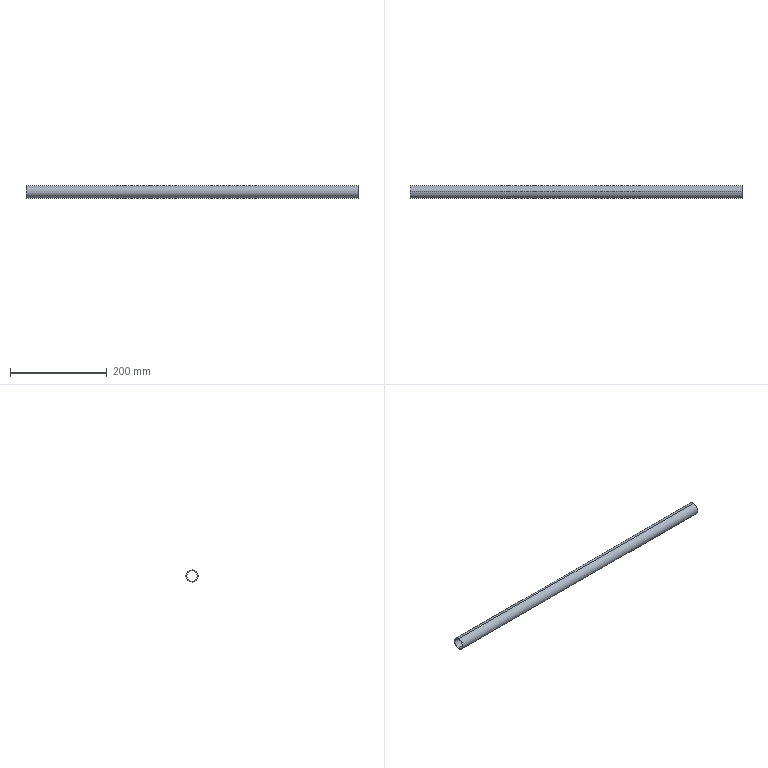Part | STEP file | E3-中转釜护栏7栏杆_Default<As Machined> | 1 solid | 6 faces | box 685 x 25 x 25 mm | volume 75858 mm3 | cylinder 4 | plane 2 | commonest cylinder face diameters 22 x2 25 x2
STEP:
#1=CARTESIAN_POINT('',(0.,0.,0.));
#2=DIRECTION('',(0.,0.,1.));
#3=DIRECTION('',(1.,0.,0.));
#4=AXIS2_PLACEMENT_3D('',#1,#2,#3);
#5=CARTESIAN_POINT('',(0.,0.,-12.5));
#6=VERTEX_POINT('',#5);
#7=CARTESIAN_POINT('',(0.,0.,12.5));
#8=VERTEX_POINT('',#7);
#9=CARTESIAN_POINT('',(0.,0.,0.));
#10=DIRECTION('',(-1.,0.,0.));
#11=DIRECTION('',(0.,0.,1.));
#12=AXIS2_PLACEMENT_3D('',#9,#10,#11);
#13=CIRCLE('',#12,12.5);
#14=CARTESIAN_POINT('',(0.,0.,0.));
#15=DIRECTION('',(-1.,0.,0.));
#16=DIRECTION('',(0.,0.,-1.));
#17=AXIS2_PLACEMENT_3D('',#14,#15,#16);
#18=CYLINDRICAL_SURFACE('',#17,12.5);
#19=CARTESIAN_POINT('',(-3.142,0.));
#20=DIRECTION('',(1.,0.));
#21=VECTOR('',#20,1.);
#22=LINE('',#19,#21);
#23=(GEOMETRIC_REPRESENTATION_CONTEXT(2)PARAMETRIC_REPRESENTATION_CONTEXT()REPRESENTATION_CONTEXT('',''));
#24=DEFINITIONAL_REPRESENTATION('',(#22),#23);
#25=PCURVE('',#18,#24);
#26=CARTESIAN_POINT('',(0.,0.,0.));
#27=DIRECTION('',(1.,0.,0.));
#28=DIRECTION('',(0.,0.,1.));
#29=AXIS2_PLACEMENT_3D('',#26,#27,#28);
#30=PLANE('',#29);
#31=CARTESIAN_POINT('',(12.5,0.));
#32=CARTESIAN_POINT('',(12.5,-21.651));
#33=CARTESIAN_POINT('',(-6.25,-10.825));
#34=CARTESIAN_POINT('',(-25.,0.));
#35=CARTESIAN_POINT('',(-6.25,10.825));
#36=CARTESIAN_POINT('',(12.5,21.651));
#37=CARTESIAN_POINT('',(12.5,0.));
#38=(BOUNDED_CURVE()B_SPLINE_CURVE(2,(#31,#32,#33,#34,#35,#36,#37),.UNSPECIFIED.,.T.,.F.)B_SPLINE_CURVE_WITH_KNOTS((1,2,2,2,2,1),(-2.094,0.,2.094,4.189,6.283,8.378),.UNSPECIFIED.)CURVE()GEOMETRIC_REPRESENTATION_ITEM()RATIONAL_B_SPLINE_CURVE((1.,0.5,1.,0.5,1.,0.5,1.))REPRESENTATION_ITEM(''));
#39=(GEOMETRIC_REPRESENTATION_CONTEXT(2)PARAMETRIC_REPRESENTATION_CONTEXT()REPRESENTATION_CONTEXT('',''));
#40=DEFINITIONAL_REPRESENTATION('',(#38),#39);
#41=PCURVE('',#30,#40);
#42=SURFACE_CURVE('',#13,(#25,#41),.PCURVE_S1.);
#43=EDGE_CURVE('',#6,#8,#42,.T.);
#44=ORIENTED_EDGE('',*,*,#43,.T.);
#45=CARTESIAN_POINT('',(-685.,0.,12.5));
#46=VERTEX_POINT('',#45);
#47=CARTESIAN_POINT('',(0.,0.,12.5));
#48=DIRECTION('',(-1.,0.,0.));
#49=VECTOR('',#48,1.);
#50=LINE('',#47,#49);
#51=CARTESIAN_POINT('',(3.142,0.));
#52=DIRECTION('',(0.,1.));
#53=VECTOR('',#52,1.);
#54=LINE('',#51,#53);
#55=(GEOMETRIC_REPRESENTATION_CONTEXT(2)PARAMETRIC_REPRESENTATION_CONTEXT()REPRESENTATION_CONTEXT('',''));
#56=DEFINITIONAL_REPRESENTATION('',(#54),#55);
#57=PCURVE('',#18,#56);
#58=CARTESIAN_POINT('',(0.,0.,0.));
#59=DIRECTION('',(-1.,0.,0.));
#60=DIRECTION('',(0.,0.,-1.));
#61=AXIS2_PLACEMENT_3D('',#58,#59,#60);
#62=CYLINDRICAL_SURFACE('',#61,12.5);
#63=CARTESIAN_POINT('',(3.142,0.));
#64=DIRECTION('',(0.,1.));
#65=VECTOR('',#64,1.);
#66=LINE('',#63,#65);
#67=(GEOMETRIC_REPRESENTATION_CONTEXT(2)PARAMETRIC_REPRESENTATION_CONTEXT()REPRESENTATION_CONTEXT('',''));
#68=DEFINITIONAL_REPRESENTATION('',(#66),#67);
#69=PCURVE('',#62,#68);
#70=SURFACE_CURVE('',#50,(#57,#69),.PCURVE_S1.);
#71=EDGE_CURVE('',#8,#46,#70,.T.);
#72=ORIENTED_EDGE('',*,*,#71,.T.);
#73=CARTESIAN_POINT('',(-685.,0.,-12.5));
#74=VERTEX_POINT('',#73);
#75=CARTESIAN_POINT('',(-685.,0.,0.));
#76=DIRECTION('',(-1.,0.,0.));
#77=DIRECTION('',(0.,0.,1.));
#78=AXIS2_PLACEMENT_3D('',#75,#76,#77);
#79=CIRCLE('',#78,12.5);
#80=CARTESIAN_POINT('',(-3.142,685.));
#81=DIRECTION('',(1.,0.));
#82=VECTOR('',#81,1.);
#83=LINE('',#80,#82);
#84=(GEOMETRIC_REPRESENTATION_CONTEXT(2)PARAMETRIC_REPRESENTATION_CONTEXT()REPRESENTATION_CONTEXT('',''));
#85=DEFINITIONAL_REPRESENTATION('',(#83),#84);
#86=PCURVE('',#18,#85);
#87=CARTESIAN_POINT('',(-685.,0.,0.));
#88=DIRECTION('',(1.,0.,0.));
#89=DIRECTION('',(0.,0.,1.));
#90=AXIS2_PLACEMENT_3D('',#87,#88,#89);
#91=PLANE('',#90);
#92=CARTESIAN_POINT('',(12.5,0.));
#93=CARTESIAN_POINT('',(12.5,-21.651));
#94=CARTESIAN_POINT('',(-6.25,-10.825));
#95=CARTESIAN_POINT('',(-25.,0.));
#96=CARTESIAN_POINT('',(-6.25,10.825));
#97=CARTESIAN_POINT('',(12.5,21.651));
#98=CARTESIAN_POINT('',(12.5,0.));
#99=(BOUNDED_CURVE()B_SPLINE_CURVE(2,(#92,#93,#94,#95,#96,#97,#98),.UNSPECIFIED.,.T.,.F.)B_SPLINE_CURVE_WITH_KNOTS((1,2,2,2,2,1),(-2.094,0.,2.094,4.189,6.283,8.378),.UNSPECIFIED.)CURVE()GEOMETRIC_REPRESENTATION_ITEM()RATIONAL_B_SPLINE_CURVE((1.,0.5,1.,0.5,1.,0.5,1.))REPRESENTATION_ITEM(''));
#100=(GEOMETRIC_REPRESENTATION_CONTEXT(2)PARAMETRIC_REPRESENTATION_CONTEXT()REPRESENTATION_CONTEXT('',''));
#101=DEFINITIONAL_REPRESENTATION('',(#99),#100);
#102=PCURVE('',#91,#101);
#103=SURFACE_CURVE('',#79,(#86,#102),.PCURVE_S1.);
#104=EDGE_CURVE('',#74,#46,#103,.T.);
#105=ORIENTED_EDGE('',*,*,#104,.F.);
#106=CARTESIAN_POINT('',(0.,0.,-12.5));
#107=DIRECTION('',(-1.,0.,0.));
#108=VECTOR('',#107,1.);
#109=LINE('',#106,#108);
#110=CARTESIAN_POINT('',(0.,0.));
#111=DIRECTION('',(0.,1.));
#112=VECTOR('',#111,1.);
#113=LINE('',#110,#112);
#114=(GEOMETRIC_REPRESENTATION_CONTEXT(2)PARAMETRIC_REPRESENTATION_CONTEXT()REPRESENTATION_CONTEXT('',''));
#115=DEFINITIONAL_REPRESENTATION('',(#113),#114);
#116=PCURVE('',#18,#115);
#117=CARTESIAN_POINT('',(6.283,0.));
#118=DIRECTION('',(0.,1.));
#119=VECTOR('',#118,1.);
#120=LINE('',#117,#119);
#121=(GEOMETRIC_REPRESENTATION_CONTEXT(2)PARAMETRIC_REPRESENTATION_CONTEXT()REPRESENTATION_CONTEXT('',''));
#122=DEFINITIONAL_REPRESENTATION('',(#120),#121);
#123=PCURVE('',#62,#122);
#124=SURFACE_CURVE('',#109,(#116,#123),.PCURVE_S1.);
#125=EDGE_CURVE('',#6,#74,#124,.T.);
#126=ORIENTED_EDGE('',*,*,#125,.F.);
#127=EDGE_LOOP('',(#44,#72,#105,#126));
#128=FACE_BOUND('',#127,.T.);
#129=ADVANCED_FACE('',(#128),#18,.T.);
#130=CARTESIAN_POINT('',(0.,0.,-11.));
#131=VERTEX_POINT('',#130);
#132=CARTESIAN_POINT('',(-685.,0.,-11.));
#133=VERTEX_POINT('',#132);
#134=CARTESIAN_POINT('',(0.,0.,-11.));
#135=DIRECTION('',(-1.,0.,0.));
#136=VECTOR('',#135,1.);
#137=LINE('',#134,#136);
#138=CARTESIAN_POINT('',(0.,0.,0.));
#139=DIRECTION('',(-1.,0.,0.));
#140=DIRECTION('',(0.,0.,-1.));
#141=AXIS2_PLACEMENT_3D('',#138,#139,#140);
#142=CYLINDRICAL_SURFACE('',#141,11.);
#143=CARTESIAN_POINT('',(6.283,0.));
#144=DIRECTION('',(0.,1.));
#145=VECTOR('',#144,1.);
#146=LINE('',#143,#145);
#147=(GEOMETRIC_REPRESENTATION_CONTEXT(2)PARAMETRIC_REPRESENTATION_CONTEXT()REPRESENTATION_CONTEXT('',''));
#148=DEFINITIONAL_REPRESENTATION('',(#146),#147);
#149=PCURVE('',#142,#148);
#150=CARTESIAN_POINT('',(0.,0.,0.));
#151=DIRECTION('',(-1.,0.,0.));
#152=DIRECTION('',(0.,0.,-1.));
#153=AXIS2_PLACEMENT_3D('',#150,#151,#152);
#154=CYLINDRICAL_SURFACE('',#153,11.);
#155=CARTESIAN_POINT('',(0.,0.));
#156=DIRECTION('',(0.,1.));
#157=VECTOR('',#156,1.);
#158=LINE('',#155,#157);
#159=(GEOMETRIC_REPRESENTATION_CONTEXT(2)PARAMETRIC_REPRESENTATION_CONTEXT()REPRESENTATION_CONTEXT('',''));
#160=DEFINITIONAL_REPRESENTATION('',(#158),#159);
#161=PCURVE('',#154,#160);
#162=SURFACE_CURVE('',#137,(#149,#161),.PCURVE_S1.);
#163=EDGE_CURVE('',#131,#133,#162,.T.);
#164=ORIENTED_EDGE('',*,*,#163,.T.);
#165=CARTESIAN_POINT('',(-685.,0.,11.));
#166=VERTEX_POINT('',#165);
#167=CARTESIAN_POINT('',(-685.,0.,0.));
#168=DIRECTION('',(-1.,0.,0.));
#169=DIRECTION('',(0.,0.,1.));
#170=AXIS2_PLACEMENT_3D('',#167,#168,#169);
#171=CIRCLE('',#170,11.);
#172=CARTESIAN_POINT('',(3.142,685.));
#173=DIRECTION('',(1.,0.));
#174=VECTOR('',#173,1.);
#175=LINE('',#172,#174);
#176=(GEOMETRIC_REPRESENTATION_CONTEXT(2)PARAMETRIC_REPRESENTATION_CONTEXT()REPRESENTATION_CONTEXT('',''));
#177=DEFINITIONAL_REPRESENTATION('',(#175),#176);
#178=PCURVE('',#142,#177);
#179=CARTESIAN_POINT('',(11.,0.));
#180=CARTESIAN_POINT('',(11.,-19.053));
#181=CARTESIAN_POINT('',(-5.5,-9.526));
#182=CARTESIAN_POINT('',(-22.,0.));
#183=CARTESIAN_POINT('',(-5.5,9.526));
#184=CARTESIAN_POINT('',(11.,19.053));
#185=CARTESIAN_POINT('',(11.,0.));
#186=(BOUNDED_CURVE()B_SPLINE_CURVE(2,(#179,#180,#181,#182,#183,#184,#185),.UNSPECIFIED.,.T.,.F.)B_SPLINE_CURVE_WITH_KNOTS((1,2,2,2,2,1),(-2.094,0.,2.094,4.189,6.283,8.378),.UNSPECIFIED.)CURVE()GEOMETRIC_REPRESENTATION_ITEM()RATIONAL_B_SPLINE_CURVE((1.,0.5,1.,0.5,1.,0.5,1.))REPRESENTATION_ITEM(''));
#187=(GEOMETRIC_REPRESENTATION_CONTEXT(2)PARAMETRIC_REPRESENTATION_CONTEXT()REPRESENTATION_CONTEXT('',''));
#188=DEFINITIONAL_REPRESENTATION('',(#186),#187);
#189=PCURVE('',#91,#188);
#190=SURFACE_CURVE('',#171,(#178,#189),.PCURVE_S1.);
#191=EDGE_CURVE('',#166,#133,#190,.T.);
#192=ORIENTED_EDGE('',*,*,#191,.F.);
#193=CARTESIAN_POINT('',(0.,0.,11.));
#194=VERTEX_POINT('',#193);
#195=CARTESIAN_POINT('',(0.,0.,11.));
#196=DIRECTION('',(-1.,0.,0.));
#197=VECTOR('',#196,1.);
#198=LINE('',#195,#197);
#199=CARTESIAN_POINT('',(3.142,0.));
#200=DIRECTION('',(0.,1.));
#201=VECTOR('',#200,1.);
#202=LINE('',#199,#201);
#203=(GEOMETRIC_REPRESENTATION_CONTEXT(2)PARAMETRIC_REPRESENTATION_CONTEXT()REPRESENTATION_CONTEXT('',''));
#204=DEFINITIONAL_REPRESENTATION('',(#202),#203);
#205=PCURVE('',#142,#204);
#206=CARTESIAN_POINT('',(3.142,0.));
#207=DIRECTION('',(0.,1.));
#208=VECTOR('',#207,1.);
#209=LINE('',#206,#208);
#210=(GEOMETRIC_REPRESENTATION_CONTEXT(2)PARAMETRIC_REPRESENTATION_CONTEXT()REPRESENTATION_CONTEXT('',''));
#211=DEFINITIONAL_REPRESENTATION('',(#209),#210);
#212=PCURVE('',#154,#211);
#213=SURFACE_CURVE('',#198,(#205,#212),.PCURVE_S1.);
#214=EDGE_CURVE('',#194,#166,#213,.T.);
#215=ORIENTED_EDGE('',*,*,#214,.F.);
#216=CARTESIAN_POINT('',(0.,0.,0.));
#217=DIRECTION('',(-1.,0.,0.));
#218=DIRECTION('',(0.,0.,1.));
#219=AXIS2_PLACEMENT_3D('',#216,#217,#218);
#220=CIRCLE('',#219,11.);
#221=CARTESIAN_POINT('',(3.142,0.));
#222=DIRECTION('',(1.,0.));
#223=VECTOR('',#222,1.);
#224=LINE('',#221,#223);
#225=(GEOMETRIC_REPRESENTATION_CONTEXT(2)PARAMETRIC_REPRESENTATION_CONTEXT()REPRESENTATION_CONTEXT('',''));
#226=DEFINITIONAL_REPRESENTATION('',(#224),#225);
#227=PCURVE('',#142,#226);
#228=CARTESIAN_POINT('',(11.,0.));
#229=CARTESIAN_POINT('',(11.,-19.053));
#230=CARTESIAN_POINT('',(-5.5,-9.526));
#231=CARTESIAN_POINT('',(-22.,0.));
#232=CARTESIAN_POINT('',(-5.5,9.526));
#233=CARTESIAN_POINT('',(11.,19.053));
#234=CARTESIAN_POINT('',(11.,0.));
#235=(BOUNDED_CURVE()B_SPLINE_CURVE(2,(#228,#229,#230,#231,#232,#233,#234),.UNSPECIFIED.,.T.,.F.)B_SPLINE_CURVE_WITH_KNOTS((1,2,2,2,2,1),(-2.094,0.,2.094,4.189,6.283,8.378),.UNSPECIFIED.)CURVE()GEOMETRIC_REPRESENTATION_ITEM()RATIONAL_B_SPLINE_CURVE((1.,0.5,1.,0.5,1.,0.5,1.))REPRESENTATION_ITEM(''));
#236=(GEOMETRIC_REPRESENTATION_CONTEXT(2)PARAMETRIC_REPRESENTATION_CONTEXT()REPRESENTATION_CONTEXT('',''));
#237=DEFINITIONAL_REPRESENTATION('',(#235),#236);
#238=PCURVE('',#30,#237);
#239=SURFACE_CURVE('',#220,(#227,#238),.PCURVE_S1.);
#240=EDGE_CURVE('',#194,#131,#239,.T.);
#241=ORIENTED_EDGE('',*,*,#240,.T.);
#242=EDGE_LOOP('',(#164,#192,#215,#241));
#243=FACE_BOUND('',#242,.F.);
#244=ADVANCED_FACE('',(#243),#142,.F.);
#245=CARTESIAN_POINT('',(-685.,0.,0.));
#246=DIRECTION('',(-1.,0.,0.));
#247=DIRECTION('',(0.,0.,1.));
#248=AXIS2_PLACEMENT_3D('',#245,#246,#247);
#249=CIRCLE('',#248,11.);
#250=CARTESIAN_POINT('',(-3.142,685.));
#251=DIRECTION('',(1.,0.));
#252=VECTOR('',#251,1.);
#253=LINE('',#250,#252);
#254=(GEOMETRIC_REPRESENTATION_CONTEXT(2)PARAMETRIC_REPRESENTATION_CONTEXT()REPRESENTATION_CONTEXT('',''));
#255=DEFINITIONAL_REPRESENTATION('',(#253),#254);
#256=PCURVE('',#154,#255);
#257=CARTESIAN_POINT('',(11.,0.));
#258=CARTESIAN_POINT('',(11.,-19.053));
#259=CARTESIAN_POINT('',(-5.5,-9.526));
#260=CARTESIAN_POINT('',(-22.,0.));
#261=CARTESIAN_POINT('',(-5.5,9.526));
#262=CARTESIAN_POINT('',(11.,19.053));
#263=CARTESIAN_POINT('',(11.,0.));
#264=(BOUNDED_CURVE()B_SPLINE_CURVE(2,(#257,#258,#259,#260,#261,#262,#263),.UNSPECIFIED.,.T.,.F.)B_SPLINE_CURVE_WITH_KNOTS((1,2,2,2,2,1),(-2.094,0.,2.094,4.189,6.283,8.378),.UNSPECIFIED.)CURVE()GEOMETRIC_REPRESENTATION_ITEM()RATIONAL_B_SPLINE_CURVE((1.,0.5,1.,0.5,1.,0.5,1.))REPRESENTATION_ITEM(''));
#265=(GEOMETRIC_REPRESENTATION_CONTEXT(2)PARAMETRIC_REPRESENTATION_CONTEXT()REPRESENTATION_CONTEXT('',''));
#266=DEFINITIONAL_REPRESENTATION('',(#264),#265);
#267=PCURVE('',#91,#266);
#268=SURFACE_CURVE('',#249,(#256,#267),.PCURVE_S1.);
#269=EDGE_CURVE('',#133,#166,#268,.T.);
#270=ORIENTED_EDGE('',*,*,#269,.F.);
#271=ORIENTED_EDGE('',*,*,#163,.F.);
#272=CARTESIAN_POINT('',(0.,0.,0.));
#273=DIRECTION('',(-1.,0.,0.));
#274=DIRECTION('',(0.,0.,1.));
#275=AXIS2_PLACEMENT_3D('',#272,#273,#274);
#276=CIRCLE('',#275,11.);
#277=CARTESIAN_POINT('',(-3.142,0.));
#278=DIRECTION('',(1.,0.));
#279=VECTOR('',#278,1.);
#280=LINE('',#277,#279);
#281=(GEOMETRIC_REPRESENTATION_CONTEXT(2)PARAMETRIC_REPRESENTATION_CONTEXT()REPRESENTATION_CONTEXT('',''));
#282=DEFINITIONAL_REPRESENTATION('',(#280),#281);
#283=PCURVE('',#154,#282);
#284=CARTESIAN_POINT('',(11.,0.));
#285=CARTESIAN_POINT('',(11.,-19.053));
#286=CARTESIAN_POINT('',(-5.5,-9.526));
#287=CARTESIAN_POINT('',(-22.,0.));
#288=CARTESIAN_POINT('',(-5.5,9.526));
#289=CARTESIAN_POINT('',(11.,19.053));
#290=CARTESIAN_POINT('',(11.,0.));
#291=(BOUNDED_CURVE()B_SPLINE_CURVE(2,(#284,#285,#286,#287,#288,#289,#290),.UNSPECIFIED.,.T.,.F.)B_SPLINE_CURVE_WITH_KNOTS((1,2,2,2,2,1),(-2.094,0.,2.094,4.189,6.283,8.378),.UNSPECIFIED.)CURVE()GEOMETRIC_REPRESENTATION_ITEM()RATIONAL_B_SPLINE_CURVE((1.,0.5,1.,0.5,1.,0.5,1.))REPRESENTATION_ITEM(''));
#292=(GEOMETRIC_REPRESENTATION_CONTEXT(2)PARAMETRIC_REPRESENTATION_CONTEXT()REPRESENTATION_CONTEXT('',''));
#293=DEFINITIONAL_REPRESENTATION('',(#291),#292);
#294=PCURVE('',#30,#293);
#295=SURFACE_CURVE('',#276,(#283,#294),.PCURVE_S1.);
#296=EDGE_CURVE('',#131,#194,#295,.T.);
#297=ORIENTED_EDGE('',*,*,#296,.T.);
#298=ORIENTED_EDGE('',*,*,#214,.T.);
#299=EDGE_LOOP('',(#270,#271,#297,#298));
#300=FACE_BOUND('',#299,.F.);
#301=ADVANCED_FACE('',(#300),#154,.F.);
#302=ORIENTED_EDGE('',*,*,#71,.F.);
#303=CARTESIAN_POINT('',(0.,0.,0.));
#304=DIRECTION('',(-1.,0.,0.));
#305=DIRECTION('',(0.,0.,1.));
#306=AXIS2_PLACEMENT_3D('',#303,#304,#305);
#307=CIRCLE('',#306,12.5);
#308=CARTESIAN_POINT('',(3.142,0.));
#309=DIRECTION('',(1.,0.));
#310=VECTOR('',#309,1.);
#311=LINE('',#308,#310);
#312=(GEOMETRIC_REPRESENTATION_CONTEXT(2)PARAMETRIC_REPRESENTATION_CONTEXT()REPRESENTATION_CONTEXT('',''));
#313=DEFINITIONAL_REPRESENTATION('',(#311),#312);
#314=PCURVE('',#62,#313);
#315=CARTESIAN_POINT('',(12.5,0.));
#316=CARTESIAN_POINT('',(12.5,-21.651));
#317=CARTESIAN_POINT('',(-6.25,-10.825));
#318=CARTESIAN_POINT('',(-25.,0.));
#319=CARTESIAN_POINT('',(-6.25,10.825));
#320=CARTESIAN_POINT('',(12.5,21.651));
#321=CARTESIAN_POINT('',(12.5,0.));
#322=(BOUNDED_CURVE()B_SPLINE_CURVE(2,(#315,#316,#317,#318,#319,#320,#321),.UNSPECIFIED.,.T.,.F.)B_SPLINE_CURVE_WITH_KNOTS((1,2,2,2,2,1),(-2.094,0.,2.094,4.189,6.283,8.378),.UNSPECIFIED.)CURVE()GEOMETRIC_REPRESENTATION_ITEM()RATIONAL_B_SPLINE_CURVE((1.,0.5,1.,0.5,1.,0.5,1.))REPRESENTATION_ITEM(''));
#323=(GEOMETRIC_REPRESENTATION_CONTEXT(2)PARAMETRIC_REPRESENTATION_CONTEXT()REPRESENTATION_CONTEXT('',''));
#324=DEFINITIONAL_REPRESENTATION('',(#322),#323);
#325=PCURVE('',#30,#324);
#326=SURFACE_CURVE('',#307,(#314,#325),.PCURVE_S1.);
#327=EDGE_CURVE('',#8,#6,#326,.T.);
#328=ORIENTED_EDGE('',*,*,#327,.T.);
#329=ORIENTED_EDGE('',*,*,#125,.T.);
#330=CARTESIAN_POINT('',(-685.,0.,0.));
#331=DIRECTION('',(-1.,0.,0.));
#332=DIRECTION('',(0.,0.,1.));
#333=AXIS2_PLACEMENT_3D('',#330,#331,#332);
#334=CIRCLE('',#333,12.5);
#335=CARTESIAN_POINT('',(3.142,685.));
#336=DIRECTION('',(1.,0.));
#337=VECTOR('',#336,1.);
#338=LINE('',#335,#337);
#339=(GEOMETRIC_REPRESENTATION_CONTEXT(2)PARAMETRIC_REPRESENTATION_CONTEXT()REPRESENTATION_CONTEXT('',''));
#340=DEFINITIONAL_REPRESENTATION('',(#338),#339);
#341=PCURVE('',#62,#340);
#342=CARTESIAN_POINT('',(12.5,0.));
#343=CARTESIAN_POINT('',(12.5,-21.651));
#344=CARTESIAN_POINT('',(-6.25,-10.825));
#345=CARTESIAN_POINT('',(-25.,0.));
#346=CARTESIAN_POINT('',(-6.25,10.825));
#347=CARTESIAN_POINT('',(12.5,21.651));
#348=CARTESIAN_POINT('',(12.5,0.));
#349=(BOUNDED_CURVE()B_SPLINE_CURVE(2,(#342,#343,#344,#345,#346,#347,#348),.UNSPECIFIED.,.T.,.F.)B_SPLINE_CURVE_WITH_KNOTS((1,2,2,2,2,1),(-2.094,0.,2.094,4.189,6.283,8.378),.UNSPECIFIED.)CURVE()GEOMETRIC_REPRESENTATION_ITEM()RATIONAL_B_SPLINE_CURVE((1.,0.5,1.,0.5,1.,0.5,1.))REPRESENTATION_ITEM(''));
#350=(GEOMETRIC_REPRESENTATION_CONTEXT(2)PARAMETRIC_REPRESENTATION_CONTEXT()REPRESENTATION_CONTEXT('',''));
#351=DEFINITIONAL_REPRESENTATION('',(#349),#350);
#352=PCURVE('',#91,#351);
#353=SURFACE_CURVE('',#334,(#341,#352),.PCURVE_S1.);
#354=EDGE_CURVE('',#46,#74,#353,.T.);
#355=ORIENTED_EDGE('',*,*,#354,.F.);
#356=EDGE_LOOP('',(#302,#328,#329,#355));
#357=FACE_BOUND('',#356,.T.);
#358=ADVANCED_FACE('',(#357),#62,.T.);
#359=ORIENTED_EDGE('',*,*,#296,.T.);
#360=ORIENTED_EDGE('',*,*,#240,.T.);
#361=EDGE_LOOP('',(#359,#360));
#362=FACE_BOUND('',#361,.T.);
#363=ORIENTED_EDGE('',*,*,#43,.F.);
#364=ORIENTED_EDGE('',*,*,#327,.F.);
#365=EDGE_LOOP('',(#363,#364));
#366=FACE_BOUND('',#365,.T.);
#367=ADVANCED_FACE('',(#362,#366),#30,.T.);
#368=ORIENTED_EDGE('',*,*,#269,.F.);
#369=ORIENTED_EDGE('',*,*,#191,.F.);
#370=EDGE_LOOP('',(#368,#369));
#371=FACE_BOUND('',#370,.T.);
#372=ORIENTED_EDGE('',*,*,#104,.T.);
#373=ORIENTED_EDGE('',*,*,#354,.T.);
#374=EDGE_LOOP('',(#372,#373));
#375=FACE_BOUND('',#374,.T.);
#376=ADVANCED_FACE('',(#371,#375),#91,.F.);
#377=CLOSED_SHELL('',(#129,#244,#301,#358,#367,#376));
#378=MANIFOLD_SOLID_BREP('',#377);
#379=(LENGTH_UNIT()NAMED_UNIT(*)SI_UNIT(.MILLI.,.METRE.));
#380=UNCERTAINTY_MEASURE_WITH_UNIT(LENGTH_MEASURE(0.0000001),#379,'','');
#381=(NAMED_UNIT(*)PLANE_ANGLE_UNIT()SI_UNIT($,.RADIAN.));
#382=(NAMED_UNIT(*)SI_UNIT($,.STERADIAN.)SOLID_ANGLE_UNIT());
#383=(GEOMETRIC_REPRESENTATION_CONTEXT(3)GLOBAL_UNCERTAINTY_ASSIGNED_CONTEXT((#380))GLOBAL_UNIT_ASSIGNED_CONTEXT((#379,#381,#382))REPRESENTATION_CONTEXT('',''));
#384=ADVANCED_BREP_SHAPE_REPRESENTATION('',(#4,#378),#383);